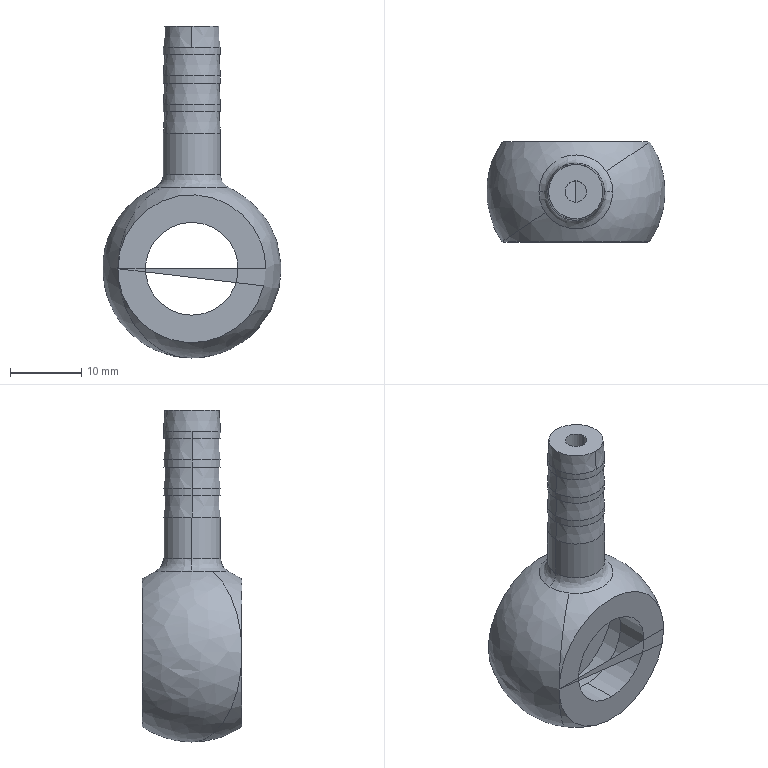Part | SolidWorks | features BaseBody 1 | 1 solid | 37 faces | box 25 x 14 x 46.5 mm | volume 4501 mm3 | cylinder 16 | plane 9 | cone 8 | spline 4 | commonest cylinder face diameters 8 x8 13 x4 3 x2 19 x2
STEP:
#1=CARTESIAN_POINT('',(0.,0.,-12.5));
#2=VERTEX_POINT('',#1);
#3=CARTESIAN_POINT('',(-10.356,-7.,0.));
#4=VERTEX_POINT('',#3);
#5=CARTESIAN_POINT('',(0.,0.,0.));
#6=DIRECTION('',(-0.56,0.8285,0.));
#7=DIRECTION('',(0.,0.,-1.));
#8=AXIS2_PLACEMENT_3D('',#5,#6,#7);
#9=CIRCLE('',#8,12.5);
#10=EDGE_CURVE('',#2,#4,#9,.T.);
#11=ORIENTED_EDGE('',*,*,#10,.F.);
#12=CARTESIAN_POINT('',(10.356,7.,0.));
#13=VERTEX_POINT('',#12);
#14=CARTESIAN_POINT('',(0.,0.,0.));
#15=DIRECTION('',(0.56,-0.8285,0.));
#16=DIRECTION('',(0.,0.,-1.));
#17=AXIS2_PLACEMENT_3D('',#14,#15,#16);
#18=CIRCLE('',#17,12.5);
#19=EDGE_CURVE('',#2,#13,#18,.T.);
#20=ORIENTED_EDGE('',*,*,#19,.T.);
#21=CARTESIAN_POINT('',(4.285,2.897,11.38));
#22=VERTEX_POINT('',#21);
#23=CARTESIAN_POINT('',(0.,0.,0.));
#24=DIRECTION('',(0.56,-0.8285,0.));
#25=DIRECTION('',(0.,0.,-1.));
#26=AXIS2_PLACEMENT_3D('',#23,#24,#25);
#27=CIRCLE('',#26,12.5);
#28=EDGE_CURVE('',#13,#22,#27,.T.);
#29=ORIENTED_EDGE('',*,*,#28,.T.);
#30=CARTESIAN_POINT('',(5.172,-0.000001778,11.38));
#31=VERTEX_POINT('',#30);
#32=CARTESIAN_POINT('',(4.285,2.897,11.38));
#33=CARTESIAN_POINT('',(4.572,2.472,11.38));
#34=CARTESIAN_POINT('',(4.796,2.005,11.38));
#35=CARTESIAN_POINT('',(5.096,1.025,11.38));
#36=CARTESIAN_POINT('',(5.172,0.5124,11.38));
#37=CARTESIAN_POINT('',(5.172,-0.000001778,11.38));
#38=B_SPLINE_CURVE_WITH_KNOTS('',3,(#32,#33,#34,#35,#36,#37),.UNSPECIFIED.,.F.,.F.,(4,2,4),(0.7255,0.8627,1.),.UNSPECIFIED.);
#39=EDGE_CURVE('',#22,#31,#38,.T.);
#40=ORIENTED_EDGE('',*,*,#39,.T.);
#41=CARTESIAN_POINT('',(2.897,-4.285,11.38));
#42=VERTEX_POINT('',#41);
#43=CARTESIAN_POINT('',(0.,0.,11.38));
#44=DIRECTION('',(0.,0.,-1.));
#45=DIRECTION('',(-0.8285,-0.56,0.));
#46=AXIS2_PLACEMENT_3D('',#43,#44,#45);
#47=CIRCLE('',#46,5.172);
#48=EDGE_CURVE('',#31,#42,#47,.T.);
#49=ORIENTED_EDGE('',*,*,#48,.T.);
#50=CARTESIAN_POINT('',(-4.285,-2.897,11.38));
#51=VERTEX_POINT('',#50);
#52=CARTESIAN_POINT('',(2.897,-4.285,11.38));
#53=CARTESIAN_POINT('',(2.336,-4.664,11.38));
#54=CARTESIAN_POINT('',(1.699,-4.932,11.38));
#55=CARTESIAN_POINT('',(0.3728,-5.203,11.38));
#56=CARTESIAN_POINT('',(-0.3172,-5.207,11.38));
#57=CARTESIAN_POINT('',(-1.647,-4.95,11.38));
#58=CARTESIAN_POINT('',(-2.286,-4.689,11.38));
#59=CARTESIAN_POINT('',(-3.416,-3.943,11.38));
#60=CARTESIAN_POINT('',(-3.906,-3.457,11.38));
#61=CARTESIAN_POINT('',(-4.285,-2.897,11.38));
#62=B_SPLINE_CURVE_WITH_KNOTS('',3,(#52,#53,#54,#55,#56,#57,#58,#59,#60,#61),.UNSPECIFIED.,.F.,.F.,(4,2,2,2,4),(0.,0.1814,0.3627,0.5441,0.7255),.UNSPECIFIED.);
#63=EDGE_CURVE('',#42,#51,#62,.T.);
#64=ORIENTED_EDGE('',*,*,#63,.T.);
#65=CARTESIAN_POINT('',(0.,0.,0.));
#66=DIRECTION('',(-0.56,0.8285,0.));
#67=DIRECTION('',(0.,0.,-1.));
#68=AXIS2_PLACEMENT_3D('',#65,#66,#67);
#69=CIRCLE('',#68,12.5);
#70=EDGE_CURVE('',#4,#51,#69,.T.);
#71=ORIENTED_EDGE('',*,*,#70,.F.);
#72=CARTESIAN_POINT('',(10.356,-7.,0.002779));
#73=VERTEX_POINT('',#72);
#74=CARTESIAN_POINT('',(-10.356,-7.,0.));
#75=CARTESIAN_POINT('',(-10.356,-7.,0.6818));
#76=CARTESIAN_POINT('',(-10.289,-7.,1.354));
#77=CARTESIAN_POINT('',(-10.092,-7.,2.347));
#78=CARTESIAN_POINT('',(-10.01,-7.,2.676));
#79=CARTESIAN_POINT('',(-9.813,-7.,3.328));
#80=CARTESIAN_POINT('',(-9.697,-7.,3.651));
#81=CARTESIAN_POINT('',(-9.308,-7.,4.589));
#82=CARTESIAN_POINT('',(-8.991,-7.,5.184));
#83=CARTESIAN_POINT('',(-8.426,-7.,6.03));
#84=CARTESIAN_POINT('',(-8.222,-7.,6.306));
#85=CARTESIAN_POINT('',(-7.79,-7.,6.832));
#86=CARTESIAN_POINT('',(-7.563,-7.,7.083));
#87=CARTESIAN_POINT('',(-6.847,-7.,7.799));
#88=CARTESIAN_POINT('',(-6.326,-7.,8.228));
#89=CARTESIAN_POINT('',(-5.19,-7.,8.988));
#90=CARTESIAN_POINT('',(-4.591,-7.,9.307));
#91=CARTESIAN_POINT('',(-3.657,-7.,9.695));
#92=CARTESIAN_POINT('',(-3.339,-7.,9.809));
#93=CARTESIAN_POINT('',(-2.689,-7.,10.007));
#94=CARTESIAN_POINT('',(-2.356,-7.,10.09));
#95=CARTESIAN_POINT('',(-1.356,-7.,10.289));
#96=CARTESIAN_POINT('',(-0.685,-7.,10.356));
#97=CARTESIAN_POINT('',(0.6675,-7.,10.357));
#98=CARTESIAN_POINT('',(1.354,-7.,10.29));
#99=CARTESIAN_POINT('',(2.68,-7.,10.026));
#100=CARTESIAN_POINT('',(3.326,-7.,9.831));
#101=CARTESIAN_POINT('',(4.269,-7.,9.442));
#102=CARTESIAN_POINT('',(4.579,-7.,9.295));
#103=CARTESIAN_POINT('',(5.181,-7.,8.973));
#104=CARTESIAN_POINT('',(5.472,-7.,8.799));
#105=CARTESIAN_POINT('',(6.314,-7.,8.236));
#106=CARTESIAN_POINT('',(6.837,-7.,7.809));
#107=CARTESIAN_POINT('',(7.56,-7.,7.086));
#108=CARTESIAN_POINT('',(7.79,-7.,6.832));
#109=CARTESIAN_POINT('',(8.22,-7.,6.309));
#110=CARTESIAN_POINT('',(8.622,-7.,5.766));
#111=CARTESIAN_POINT('',(8.97,-7.,5.187));
#112=CARTESIAN_POINT('',(9.29,-7.,4.59));
#113=CARTESIAN_POINT('',(9.436,-7.,4.28));
#114=CARTESIAN_POINT('',(9.828,-7.,3.336));
#115=CARTESIAN_POINT('',(10.023,-7.,2.69));
#116=CARTESIAN_POINT('',(10.222,-7.,1.697));
#117=CARTESIAN_POINT('',(10.272,-7.,1.362));
#118=CARTESIAN_POINT('',(10.339,-7.,0.6824));
#119=CARTESIAN_POINT('',(10.356,-7.,0.3412));
#120=CARTESIAN_POINT('',(10.356,-7.,0.002779));
#121=B_SPLINE_CURVE_WITH_KNOTS('',3,(#74,#75,#76,#77,#78,#79,#80,#81,#82,#83,#84,#85,#86,#87,#88,#89,#90,#91,#92,#93,#94,#95,#96,#97,#98,#99,#100,#101,#102,#103,#104,#105,#106,#107,#108,#109,#110,#111,#112,#113,#114,#115,#116,#117,#118,#119,#120),.UNSPECIFIED.,.F.,.F.,(4,2,2,2,2,2,2,2,2,2,2,2,2,2,2,2,2,2,1,2,2,2,2,4),(0.04367,0.04569,0.0467,0.04771,0.04974,0.05075,0.05176,0.05378,0.05581,0.05682,0.05783,0.05985,0.06188,0.0639,0.06491,0.06592,0.06795,0.06896,0.06997,0.07098,0.07199,0.07402,0.07503,0.07604),.UNSPECIFIED.);
#122=EDGE_CURVE('',#4,#73,#121,.T.);
#123=ORIENTED_EDGE('',*,*,#122,.T.);
#124=CARTESIAN_POINT('',(10.356,-7.,0.002779));
#125=CARTESIAN_POINT('',(10.356,-7.,-0.6741));
#126=CARTESIAN_POINT('',(10.291,-7.,-1.345));
#127=CARTESIAN_POINT('',(10.093,-7.,-2.344));
#128=CARTESIAN_POINT('',(10.01,-7.,-2.677));
#129=CARTESIAN_POINT('',(9.813,-7.,-3.328));
#130=CARTESIAN_POINT('',(9.699,-7.,-3.646));
#131=CARTESIAN_POINT('',(9.312,-7.,-4.582));
#132=CARTESIAN_POINT('',(8.995,-7.,-5.178));
#133=CARTESIAN_POINT('',(8.236,-7.,-6.316));
#134=CARTESIAN_POINT('',(7.806,-7.,-6.839));
#135=CARTESIAN_POINT('',(7.091,-7.,-7.555));
#136=CARTESIAN_POINT('',(6.841,-7.,-7.783));
#137=CARTESIAN_POINT('',(6.316,-7.,-8.214));
#138=CARTESIAN_POINT('',(6.041,-7.,-8.419));
#139=CARTESIAN_POINT('',(5.19,-7.,-8.988));
#140=CARTESIAN_POINT('',(4.583,-7.,-9.312));
#141=CARTESIAN_POINT('',(3.331,-7.,-9.829));
#142=CARTESIAN_POINT('',(2.686,-7.,-10.025));
#143=CARTESIAN_POINT('',(1.688,-7.,-10.223));
#144=CARTESIAN_POINT('',(1.348,-7.,-10.274));
#145=CARTESIAN_POINT('',(0.6714,-7.,-10.34));
#146=CARTESIAN_POINT('',(0.3335,-7.,-10.356));
#147=CARTESIAN_POINT('',(-0.6787,-7.,-10.356));
#148=CARTESIAN_POINT('',(-1.351,-7.,-10.29));
#149=CARTESIAN_POINT('',(-2.692,-7.,-10.023));
#150=CARTESIAN_POINT('',(-3.34,-7.,-9.826));
#151=CARTESIAN_POINT('',(-4.275,-7.,-9.439));
#152=CARTESIAN_POINT('',(-4.581,-7.,-9.294));
#153=CARTESIAN_POINT('',(-5.18,-7.,-8.974));
#154=CARTESIAN_POINT('',(-5.475,-7.,-8.797));
#155=CARTESIAN_POINT('',(-6.321,-7.,-8.231));
#156=CARTESIAN_POINT('',(-6.843,-7.,-7.803));
#157=CARTESIAN_POINT('',(-7.8,-7.,-6.847));
#158=CARTESIAN_POINT('',(-8.237,-7.,-6.313));
#159=CARTESIAN_POINT('',(-8.987,-7.,-5.19));
#160=CARTESIAN_POINT('',(-9.306,-7.,-4.595));
#161=CARTESIAN_POINT('',(-9.697,-7.,-3.652));
#162=CARTESIAN_POINT('',(-9.813,-7.,-3.329));
#163=CARTESIAN_POINT('',(-10.009,-7.,-2.68));
#164=CARTESIAN_POINT('',(-10.173,-7.,-2.024));
#165=CARTESIAN_POINT('',(-10.272,-7.,-1.357));
#166=CARTESIAN_POINT('',(-10.339,-7.,-0.6827));
#167=CARTESIAN_POINT('',(-10.356,-7.,-0.3409));
#168=CARTESIAN_POINT('',(-10.356,-7.,0.));
#169=B_SPLINE_CURVE_WITH_KNOTS('',3,(#124,#125,#126,#127,#128,#129,#130,#131,#132,#133,#134,#135,#136,#137,#138,#139,#140,#141,#142,#143,#144,#145,#146,#147,#148,#149,#150,#151,#152,#153,#154,#155,#156,#157,#158,#159,#160,#161,#162,#163,#164,#165,#166,#167,#168),.UNSPECIFIED.,.F.,.F.,(4,2,2,2,2,2,2,2,2,2,2,2,2,2,2,2,2,2,2,2,1,2,4),(0.01129,0.01332,0.01433,0.01534,0.01736,0.01939,0.0204,0.02141,0.02343,0.02546,0.02647,0.02748,0.0295,0.03153,0.03254,0.03355,0.03557,0.0376,0.03962,0.04063,0.04164,0.04265,0.04367),.UNSPECIFIED.);
#170=EDGE_CURVE('',#73,#4,#169,.T.);
#171=ORIENTED_EDGE('',*,*,#170,.T.);
#172=EDGE_LOOP('',(#11,#20,#29,#40,#49,#64,#71,#123,#171));
#173=FACE_OUTER_BOUND('',#172,.T.);
#174=CARTESIAN_POINT('',(0.,0.,-12.5));
#175=CARTESIAN_POINT('',(0.,0.,-12.5));
#176=CARTESIAN_POINT('',(0.,0.,-12.5));
#177=CARTESIAN_POINT('',(0.,0.,-12.5));
#178=CARTESIAN_POINT('',(0.,0.,-12.5));
#179=CARTESIAN_POINT('',(0.,0.,-12.5));
#180=CARTESIAN_POINT('',(0.,0.,-12.5));
#181=CARTESIAN_POINT('',(14.408,9.738,-12.5));
#182=CARTESIAN_POINT('',(20.112,1.299,-12.5));
#183=CARTESIAN_POINT('',(18.178,-8.703,-12.5));
#184=CARTESIAN_POINT('',(9.738,-14.408,-12.5));
#185=CARTESIAN_POINT('',(1.299,-20.112,-12.5));
#186=CARTESIAN_POINT('',(-8.703,-18.178,-12.5));
#187=CARTESIAN_POINT('',(-14.408,-9.738,-12.5));
#188=CARTESIAN_POINT('',(17.343,11.722,4.525));
#189=CARTESIAN_POINT('',(24.21,1.563,4.525));
#190=CARTESIAN_POINT('',(21.882,-10.476,4.525));
#191=CARTESIAN_POINT('',(11.722,-17.343,4.525));
#192=CARTESIAN_POINT('',(1.563,-24.21,4.525));
#193=CARTESIAN_POINT('',(-10.476,-21.882,4.525));
#194=CARTESIAN_POINT('',(-17.343,-11.722,4.525));
#195=CARTESIAN_POINT('',(4.131,2.792,11.462));
#196=CARTESIAN_POINT('',(5.767,0.3724,11.462));
#197=CARTESIAN_POINT('',(5.212,-2.495,11.462));
#198=CARTESIAN_POINT('',(2.792,-4.131,11.462));
#199=CARTESIAN_POINT('',(0.3724,-5.767,11.462));
#200=CARTESIAN_POINT('',(-2.495,-5.212,11.462));
#201=CARTESIAN_POINT('',(-4.131,-2.792,11.462));
#202=(BOUNDED_SURFACE()B_SPLINE_SURFACE(3,3,((#174,#175,#176,#177,#178,#179,#180),(#181,#182,#183,#184,#185,#186,#187),(#188,#189,#190,#191,#192,#193,#194),(#195,#196,#197,#198,#199,#200,#201)),.UNSPECIFIED.,.F.,.F.,.T.)B_SPLINE_SURFACE_WITH_KNOTS((4,4),(4,3,4),(0.,1.),(0.,0.5,1.),.UNSPECIFIED.)GEOMETRIC_REPRESENTATION_ITEM()RATIONAL_B_SPLINE_SURFACE(((1.,0.8047,0.8047,1.,0.8047,0.8047,1.),(0.4692,0.3775,0.3775,0.4692,0.3775,0.3775,0.4692),(0.4692,0.3775,0.3775,0.4692,0.3775,0.3775,0.4692),(1.,0.8047,0.8047,1.,0.8047,0.8047,1.)))REPRESENTATION_ITEM('')SURFACE());
#203=ADVANCED_FACE('',(#173),#202,.T.);
#204=CARTESIAN_POINT('',(-4.,0.,19.));
#205=VERTEX_POINT('',#204);
#206=CARTESIAN_POINT('',(4.,0.,19.));
#207=VERTEX_POINT('',#206);
#208=CARTESIAN_POINT('',(0.,0.,19.));
#209=DIRECTION('',(0.,0.,-1.));
#210=DIRECTION('',(-1.,0.,0.));
#211=AXIS2_PLACEMENT_3D('',#208,#209,#210);
#212=CIRCLE('',#211,4.);
#213=EDGE_CURVE('',#205,#207,#212,.T.);
#214=ORIENTED_EDGE('',*,*,#213,.T.);
#215=CARTESIAN_POINT('',(4.,-0.000001036,13.2));
#216=VERTEX_POINT('',#215);
#217=CARTESIAN_POINT('',(4.,0.,19.));
#218=DIRECTION('',(0.,0.,-1.));
#219=VECTOR('',#218,1000.);
#220=LINE('',#217,#219);
#221=EDGE_CURVE('',#207,#216,#220,.T.);
#222=ORIENTED_EDGE('',*,*,#221,.T.);
#223=CARTESIAN_POINT('',(-4.,0.000000641,13.2));
#224=VERTEX_POINT('',#223);
#225=CARTESIAN_POINT('',(-0.000000135,-0.000000379,13.2));
#226=DIRECTION('',(0.000000022,0.00000006,1.));
#227=DIRECTION('',(1.,-0.000000251,-0.000000022));
#228=AXIS2_PLACEMENT_3D('',#225,#226,#227);
#229=CIRCLE('',#228,4.);
#230=EDGE_CURVE('',#216,#224,#229,.T.);
#231=ORIENTED_EDGE('',*,*,#230,.T.);
#232=CARTESIAN_POINT('',(-4.,0.,19.));
#233=DIRECTION('',(0.,0.,-1.));
#234=VECTOR('',#233,1000.);
#235=LINE('',#232,#234);
#236=EDGE_CURVE('',#205,#224,#235,.T.);
#237=ORIENTED_EDGE('',*,*,#236,.F.);
#238=EDGE_LOOP('',(#214,#222,#231,#237));
#239=FACE_OUTER_BOUND('',#238,.T.);
#240=CARTESIAN_POINT('',(0.,0.,19.));
#241=DIRECTION('',(0.,0.,-1.));
#242=DIRECTION('',(-1.,0.,0.));
#243=AXIS2_PLACEMENT_3D('',#240,#241,#242);
#244=CYLINDRICAL_SURFACE('',#243,4.);
#245=ADVANCED_FACE('',(#239),#244,.T.);
#246=CARTESIAN_POINT('',(0.,7.,6.5));
#247=VERTEX_POINT('',#246);
#248=CARTESIAN_POINT('',(0.,7.,-6.5));
#249=VERTEX_POINT('',#248);
#250=CARTESIAN_POINT('',(0.,7.,0.));
#251=DIRECTION('',(0.,-1.,0.));
#252=DIRECTION('',(0.,0.,-1.));
#253=AXIS2_PLACEMENT_3D('',#250,#251,#252);
#254=CIRCLE('',#253,6.5);
#255=EDGE_CURVE('',#247,#249,#254,.T.);
#256=ORIENTED_EDGE('',*,*,#255,.F.);
#257=CARTESIAN_POINT('',(0.,2.333,6.5));
#258=VERTEX_POINT('',#257);
#259=CARTESIAN_POINT('',(0.,7.,6.5));
#260=DIRECTION('',(0.,-1.,0.));
#261=VECTOR('',#260,1000.);
#262=LINE('',#259,#261);
#263=EDGE_CURVE('',#247,#258,#262,.T.);
#264=ORIENTED_EDGE('',*,*,#263,.T.);
#265=CARTESIAN_POINT('',(0.,2.333,-6.5));
#266=VERTEX_POINT('',#265);
#267=CARTESIAN_POINT('',(0.,2.333,0.));
#268=DIRECTION('',(0.,1.,0.));
#269=DIRECTION('',(0.,0.,-1.));
#270=AXIS2_PLACEMENT_3D('',#267,#268,#269);
#271=CIRCLE('',#270,6.5);
#272=EDGE_CURVE('',#266,#258,#271,.T.);
#273=ORIENTED_EDGE('',*,*,#272,.F.);
#274=CARTESIAN_POINT('',(0.,7.,-6.5));
#275=DIRECTION('',(0.,-1.,0.));
#276=VECTOR('',#275,1000.);
#277=LINE('',#274,#276);
#278=EDGE_CURVE('',#249,#266,#277,.T.);
#279=ORIENTED_EDGE('',*,*,#278,.F.);
#280=EDGE_LOOP('',(#256,#264,#273,#279));
#281=FACE_OUTER_BOUND('',#280,.T.);
#282=CARTESIAN_POINT('',(0.,7.,0.));
#283=DIRECTION('',(0.,-1.,0.));
#284=DIRECTION('',(0.,0.,-1.));
#285=AXIS2_PLACEMENT_3D('',#282,#283,#284);
#286=CYLINDRICAL_SURFACE('',#285,6.5);
#287=ADVANCED_FACE('',(#281),#286,.F.);
#288=CARTESIAN_POINT('',(0.,-2.333,6.5));
#289=VERTEX_POINT('',#288);
#290=CARTESIAN_POINT('',(0.,-2.333,-6.5));
#291=VERTEX_POINT('',#290);
#292=CARTESIAN_POINT('',(0.,-2.333,0.));
#293=DIRECTION('',(0.,-1.,0.));
#294=DIRECTION('',(0.,0.,-1.));
#295=AXIS2_PLACEMENT_3D('',#292,#293,#294);
#296=CIRCLE('',#295,6.5);
#297=EDGE_CURVE('',#289,#291,#296,.T.);
#298=ORIENTED_EDGE('',*,*,#297,.F.);
#299=CARTESIAN_POINT('',(0.,-7.,6.5));
#300=VERTEX_POINT('',#299);
#301=CARTESIAN_POINT('',(0.,-2.333,6.5));
#302=DIRECTION('',(0.,-1.,0.));
#303=VECTOR('',#302,1000.);
#304=LINE('',#301,#303);
#305=EDGE_CURVE('',#289,#300,#304,.T.);
#306=ORIENTED_EDGE('',*,*,#305,.T.);
#307=CARTESIAN_POINT('',(0.,-7.,-6.5));
#308=VERTEX_POINT('',#307);
#309=CARTESIAN_POINT('',(0.,-7.,0.));
#310=DIRECTION('',(0.,-1.,0.));
#311=DIRECTION('',(0.,0.,-1.));
#312=AXIS2_PLACEMENT_3D('',#309,#310,#311);
#313=CIRCLE('',#312,6.5);
#314=EDGE_CURVE('',#300,#308,#313,.T.);
#315=ORIENTED_EDGE('',*,*,#314,.T.);
#316=CARTESIAN_POINT('',(0.,-2.333,-6.5));
#317=DIRECTION('',(0.,-1.,0.));
#318=VECTOR('',#317,1000.);
#319=LINE('',#316,#318);
#320=EDGE_CURVE('',#291,#308,#319,.T.);
#321=ORIENTED_EDGE('',*,*,#320,.F.);
#322=EDGE_LOOP('',(#298,#306,#315,#321));
#323=FACE_OUTER_BOUND('',#322,.T.);
#324=CARTESIAN_POINT('',(0.,-2.333,0.));
#325=DIRECTION('',(0.,-1.,0.));
#326=DIRECTION('',(0.,0.,-1.));
#327=AXIS2_PLACEMENT_3D('',#324,#325,#326);
#328=CYLINDRICAL_SURFACE('',#327,6.5);
#329=ADVANCED_FACE('',(#323),#328,.F.);
#330=CARTESIAN_POINT('',(-3.8,0.,22.));
#331=VERTEX_POINT('',#330);
#332=CARTESIAN_POINT('',(3.8,0.,22.));
#333=VERTEX_POINT('',#332);
#334=CARTESIAN_POINT('',(0.,0.,22.));
#335=DIRECTION('',(0.,0.,-1.));
#336=DIRECTION('',(-1.,0.,0.));
#337=AXIS2_PLACEMENT_3D('',#334,#335,#336);
#338=CIRCLE('',#337,3.8);
#339=EDGE_CURVE('',#331,#333,#338,.T.);
#340=ORIENTED_EDGE('',*,*,#339,.T.);
#341=CARTESIAN_POINT('',(4.,0.,19.));
#342=DIRECTION('',(0.06652,0.,-0.9978));
#343=VECTOR('',#342,1000.);
#344=LINE('',#341,#343);
#345=EDGE_CURVE('',#333,#207,#344,.T.);
#346=ORIENTED_EDGE('',*,*,#345,.T.);
#347=ORIENTED_EDGE('',*,*,#213,.F.);
#348=CARTESIAN_POINT('',(-4.,0.,19.));
#349=DIRECTION('',(-0.06652,0.,-0.9978));
#350=VECTOR('',#349,1000.);
#351=LINE('',#348,#350);
#352=EDGE_CURVE('',#331,#205,#351,.T.);
#353=ORIENTED_EDGE('',*,*,#352,.F.);
#354=EDGE_LOOP('',(#340,#346,#347,#353));
#355=FACE_OUTER_BOUND('',#354,.T.);
#356=CARTESIAN_POINT('',(0.,0.,19.));
#357=DIRECTION('',(0.,0.,-1.));
#358=DIRECTION('',(-1.,0.,0.));
#359=AXIS2_PLACEMENT_3D('',#356,#357,#358);
#360=CONICAL_SURFACE('',#359,4.,0.06657);
#361=ADVANCED_FACE('',(#355),#360,.T.);
#362=CARTESIAN_POINT('',(3.041,2.333,9.));
#363=VERTEX_POINT('',#362);
#364=CARTESIAN_POINT('',(0.,2.333,-9.5));
#365=VERTEX_POINT('',#364);
#366=CARTESIAN_POINT('',(0.,2.333,0.));
#367=DIRECTION('',(0.,1.,0.));
#368=DIRECTION('',(0.,0.,-1.));
#369=AXIS2_PLACEMENT_3D('',#366,#367,#368);
#370=CIRCLE('',#369,9.5);
#371=EDGE_CURVE('',#363,#365,#370,.T.);
#372=ORIENTED_EDGE('',*,*,#371,.T.);
#373=CARTESIAN_POINT('',(0.,-2.333,-9.5));
#374=VERTEX_POINT('',#373);
#375=CARTESIAN_POINT('',(0.,2.333,-9.5));
#376=DIRECTION('',(0.,-1.,0.));
#377=VECTOR('',#376,1000.);
#378=LINE('',#375,#377);
#379=EDGE_CURVE('',#365,#374,#378,.T.);
#380=ORIENTED_EDGE('',*,*,#379,.T.);
#381=CARTESIAN_POINT('',(3.041,-2.333,9.));
#382=VERTEX_POINT('',#381);
#383=CARTESIAN_POINT('',(0.,-2.333,0.));
#384=DIRECTION('',(0.,1.,0.));
#385=DIRECTION('',(0.,0.,-1.));
#386=AXIS2_PLACEMENT_3D('',#383,#384,#385);
#387=CIRCLE('',#386,9.5);
#388=EDGE_CURVE('',#382,#374,#387,.T.);
#389=ORIENTED_EDGE('',*,*,#388,.F.);
#390=CARTESIAN_POINT('',(3.041,2.333,9.));
#391=DIRECTION('',(0.,-1.,0.));
#392=VECTOR('',#391,1000.);
#393=LINE('',#390,#392);
#394=EDGE_CURVE('',#363,#382,#393,.T.);
#395=ORIENTED_EDGE('',*,*,#394,.F.);
#396=EDGE_LOOP('',(#372,#380,#389,#395));
#397=FACE_OUTER_BOUND('',#396,.T.);
#398=CARTESIAN_POINT('',(0.,2.333,0.));
#399=DIRECTION('',(0.,-1.,0.));
#400=DIRECTION('',(0.,0.,-1.));
#401=AXIS2_PLACEMENT_3D('',#398,#399,#400);
#402=CYLINDRICAL_SURFACE('',#401,9.5);
#403=ADVANCED_FACE('',(#397),#402,.F.);
#404=CARTESIAN_POINT('',(-4.,0.,23.));
#405=VERTEX_POINT('',#404);
#406=CARTESIAN_POINT('',(4.,0.,23.));
#407=VERTEX_POINT('',#406);
#408=CARTESIAN_POINT('',(0.,0.,23.));
#409=DIRECTION('',(0.,0.,-1.));
#410=DIRECTION('',(-1.,0.,0.));
#411=AXIS2_PLACEMENT_3D('',#408,#409,#410);
#412=CIRCLE('',#411,4.);
#413=EDGE_CURVE('',#405,#407,#412,.T.);
#414=ORIENTED_EDGE('',*,*,#413,.T.);
#415=CARTESIAN_POINT('',(4.,0.,22.));
#416=VERTEX_POINT('',#415);
#417=CARTESIAN_POINT('',(4.,0.,23.));
#418=DIRECTION('',(0.,0.,-1.));
#419=VECTOR('',#418,1000.);
#420=LINE('',#417,#419);
#421=EDGE_CURVE('',#407,#416,#420,.T.);
#422=ORIENTED_EDGE('',*,*,#421,.T.);
#423=CARTESIAN_POINT('',(-4.,0.,22.));
#424=VERTEX_POINT('',#423);
#425=CARTESIAN_POINT('',(0.,0.,22.));
#426=DIRECTION('',(0.,0.,1.));
#427=DIRECTION('',(-1.,0.,0.));
#428=AXIS2_PLACEMENT_3D('',#425,#426,#427);
#429=CIRCLE('',#428,4.);
#430=EDGE_CURVE('',#416,#424,#429,.T.);
#431=ORIENTED_EDGE('',*,*,#430,.T.);
#432=CARTESIAN_POINT('',(-4.,0.,23.));
#433=DIRECTION('',(0.,0.,-1.));
#434=VECTOR('',#433,1000.);
#435=LINE('',#432,#434);
#436=EDGE_CURVE('',#405,#424,#435,.T.);
#437=ORIENTED_EDGE('',*,*,#436,.F.);
#438=EDGE_LOOP('',(#414,#422,#431,#437));
#439=FACE_OUTER_BOUND('',#438,.T.);
#440=CARTESIAN_POINT('',(0.,0.,23.));
#441=DIRECTION('',(0.,0.,-1.));
#442=DIRECTION('',(-1.,0.,0.));
#443=AXIS2_PLACEMENT_3D('',#440,#441,#442);
#444=CYLINDRICAL_SURFACE('',#443,4.);
#445=ADVANCED_FACE('',(#439),#444,.T.);
#446=CARTESIAN_POINT('',(1.5,0.,34.));
#447=VERTEX_POINT('',#446);
#448=CARTESIAN_POINT('',(-1.5,0.,34.));
#449=VERTEX_POINT('',#448);
#450=CARTESIAN_POINT('',(0.,0.,34.));
#451=DIRECTION('',(0.,0.,-1.));
#452=DIRECTION('',(-1.,0.,0.));
#453=AXIS2_PLACEMENT_3D('',#450,#451,#452);
#454=CIRCLE('',#453,1.5);
#455=EDGE_CURVE('',#447,#449,#454,.T.);
#456=ORIENTED_EDGE('',*,*,#455,.F.);
#457=CARTESIAN_POINT('',(1.5,0.,9.));
#458=VERTEX_POINT('',#457);
#459=CARTESIAN_POINT('',(1.5,0.,34.));
#460=DIRECTION('',(0.,0.,-1.));
#461=VECTOR('',#460,1000.);
#462=LINE('',#459,#461);
#463=EDGE_CURVE('',#447,#458,#462,.T.);
#464=ORIENTED_EDGE('',*,*,#463,.T.);
#465=CARTESIAN_POINT('',(-1.5,0.,9.));
#466=VERTEX_POINT('',#465);
#467=CARTESIAN_POINT('',(0.,0.,9.));
#468=DIRECTION('',(0.,0.,-1.));
#469=DIRECTION('',(-1.,0.,0.));
#470=AXIS2_PLACEMENT_3D('',#467,#468,#469);
#471=CIRCLE('',#470,1.5);
#472=EDGE_CURVE('',#458,#466,#471,.T.);
#473=ORIENTED_EDGE('',*,*,#472,.T.);
#474=CARTESIAN_POINT('',(-1.5,0.,34.));
#475=DIRECTION('',(0.,0.,-1.));
#476=VECTOR('',#475,1000.);
#477=LINE('',#474,#476);
#478=EDGE_CURVE('',#449,#466,#477,.T.);
#479=ORIENTED_EDGE('',*,*,#478,.F.);
#480=EDGE_LOOP('',(#456,#464,#473,#479));
#481=FACE_OUTER_BOUND('',#480,.T.);
#482=CARTESIAN_POINT('',(0.,0.,34.));
#483=DIRECTION('',(0.,0.,-1.));
#484=DIRECTION('',(-1.,0.,0.));
#485=AXIS2_PLACEMENT_3D('',#482,#483,#484);
#486=CYLINDRICAL_SURFACE('',#485,1.5);
#487=ADVANCED_FACE('',(#481),#486,.F.);
#488=CARTESIAN_POINT('',(-3.8,0.,26.));
#489=VERTEX_POINT('',#488);
#490=CARTESIAN_POINT('',(3.8,0.,26.));
#491=VERTEX_POINT('',#490);
#492=CARTESIAN_POINT('',(0.,0.,26.));
#493=DIRECTION('',(0.,0.,-1.));
#494=DIRECTION('',(-1.,0.,0.));
#495=AXIS2_PLACEMENT_3D('',#492,#493,#494);
#496=CIRCLE('',#495,3.8);
#497=EDGE_CURVE('',#489,#491,#496,.T.);
#498=ORIENTED_EDGE('',*,*,#497,.T.);
#499=CARTESIAN_POINT('',(4.,0.,23.));
#500=DIRECTION('',(0.06652,0.,-0.9978));
#501=VECTOR('',#500,1000.);
#502=LINE('',#499,#501);
#503=EDGE_CURVE('',#491,#407,#502,.T.);
#504=ORIENTED_EDGE('',*,*,#503,.T.);
#505=ORIENTED_EDGE('',*,*,#413,.F.);
#506=CARTESIAN_POINT('',(-4.,0.,23.));
#507=DIRECTION('',(-0.06652,0.,-0.9978));
#508=VECTOR('',#507,1000.);
#509=LINE('',#506,#508);
#510=EDGE_CURVE('',#489,#405,#509,.T.);
#511=ORIENTED_EDGE('',*,*,#510,.F.);
#512=EDGE_LOOP('',(#498,#504,#505,#511));
#513=FACE_OUTER_BOUND('',#512,.T.);
#514=CARTESIAN_POINT('',(0.,0.,23.));
#515=DIRECTION('',(0.,0.,-1.));
#516=DIRECTION('',(-1.,0.,0.));
#517=AXIS2_PLACEMENT_3D('',#514,#515,#516);
#518=CONICAL_SURFACE('',#517,4.,0.06657);
#519=ADVANCED_FACE('',(#513),#518,.T.);
#520=CARTESIAN_POINT('',(0.,-3.8,34.));
#521=VERTEX_POINT('',#520);
#522=CARTESIAN_POINT('',(0.,3.8,34.));
#523=VERTEX_POINT('',#522);
#524=CARTESIAN_POINT('',(0.,0.,34.));
#525=DIRECTION('',(0.,0.,1.));
#526=DIRECTION('',(0.,1.,0.));
#527=AXIS2_PLACEMENT_3D('',#524,#525,#526);
#528=CIRCLE('',#527,3.8);
#529=EDGE_CURVE('',#521,#523,#528,.T.);
#530=ORIENTED_EDGE('',*,*,#529,.F.);
#531=CARTESIAN_POINT('',(0.,-4.,31.));
#532=VERTEX_POINT('',#531);
#533=CARTESIAN_POINT('',(0.,-4.,31.));
#534=DIRECTION('',(0.,-0.06652,-0.9978));
#535=VECTOR('',#534,1000.);
#536=LINE('',#533,#535);
#537=EDGE_CURVE('',#521,#532,#536,.T.);
#538=ORIENTED_EDGE('',*,*,#537,.T.);
#539=CARTESIAN_POINT('',(4.,0.,31.));
#540=VERTEX_POINT('',#539);
#541=CARTESIAN_POINT('',(0.,0.,31.));
#542=DIRECTION('',(0.,0.,1.));
#543=DIRECTION('',(-1.,0.,0.));
#544=AXIS2_PLACEMENT_3D('',#541,#542,#543);
#545=CIRCLE('',#544,4.);
#546=EDGE_CURVE('',#532,#540,#545,.T.);
#547=ORIENTED_EDGE('',*,*,#546,.T.);
#548=CARTESIAN_POINT('',(0.,4.,31.));
#549=VERTEX_POINT('',#548);
#550=CARTESIAN_POINT('',(0.,0.,31.));
#551=DIRECTION('',(0.,0.,1.));
#552=DIRECTION('',(-1.,0.,0.));
#553=AXIS2_PLACEMENT_3D('',#550,#551,#552);
#554=CIRCLE('',#553,4.);
#555=EDGE_CURVE('',#540,#549,#554,.T.);
#556=ORIENTED_EDGE('',*,*,#555,.T.);
#557=CARTESIAN_POINT('',(0.,4.,31.));
#558=DIRECTION('',(0.,0.06652,-0.9978));
#559=VECTOR('',#558,1000.);
#560=LINE('',#557,#559);
#561=EDGE_CURVE('',#523,#549,#560,.T.);
#562=ORIENTED_EDGE('',*,*,#561,.F.);
#563=EDGE_LOOP('',(#530,#538,#547,#556,#562));
#564=FACE_OUTER_BOUND('',#563,.T.);
#565=CARTESIAN_POINT('',(0.,0.,31.));
#566=DIRECTION('',(0.,0.,-1.));
#567=DIRECTION('',(0.,1.,0.));
#568=AXIS2_PLACEMENT_3D('',#565,#566,#567);
#569=CONICAL_SURFACE('',#568,4.,0.06657);
#570=ADVANCED_FACE('',(#564),#569,.T.);
#571=CARTESIAN_POINT('',(-4.,0.,27.));
#572=VERTEX_POINT('',#571);
#573=CARTESIAN_POINT('',(4.,0.,27.));
#574=VERTEX_POINT('',#573);
#575=CARTESIAN_POINT('',(0.,0.,27.));
#576=DIRECTION('',(0.,0.,-1.));
#577=DIRECTION('',(-1.,0.,0.));
#578=AXIS2_PLACEMENT_3D('',#575,#576,#577);
#579=CIRCLE('',#578,4.);
#580=EDGE_CURVE('',#572,#574,#579,.T.);
#581=ORIENTED_EDGE('',*,*,#580,.T.);
#582=CARTESIAN_POINT('',(4.,0.,26.));
#583=VERTEX_POINT('',#582);
#584=CARTESIAN_POINT('',(4.,0.,27.));
#585=DIRECTION('',(0.,0.,-1.));
#586=VECTOR('',#585,1000.);
#587=LINE('',#584,#586);
#588=EDGE_CURVE('',#574,#583,#587,.T.);
#589=ORIENTED_EDGE('',*,*,#588,.T.);
#590=CARTESIAN_POINT('',(-4.,0.,26.));
#591=VERTEX_POINT('',#590);
#592=CARTESIAN_POINT('',(0.,0.,26.));
#593=DIRECTION('',(0.,0.,1.));
#594=DIRECTION('',(-1.,0.,0.));
#595=AXIS2_PLACEMENT_3D('',#592,#593,#594);
#596=CIRCLE('',#595,4.);
#597=EDGE_CURVE('',#583,#591,#596,.T.);
#598=ORIENTED_EDGE('',*,*,#597,.T.);
#599=CARTESIAN_POINT('',(-4.,0.,27.));
#600=DIRECTION('',(0.,0.,-1.));
#601=VECTOR('',#600,1000.);
#602=LINE('',#599,#601);
#603=EDGE_CURVE('',#572,#591,#602,.T.);
#604=ORIENTED_EDGE('',*,*,#603,.F.);
#605=EDGE_LOOP('',(#581,#589,#598,#604));
#606=FACE_OUTER_BOUND('',#605,.T.);
#607=CARTESIAN_POINT('',(0.,0.,27.));
#608=DIRECTION('',(0.,0.,-1.));
#609=DIRECTION('',(-1.,0.,0.));
#610=AXIS2_PLACEMENT_3D('',#607,#608,#609);
#611=CYLINDRICAL_SURFACE('',#610,4.);
#612=ADVANCED_FACE('',(#606),#611,.T.);
#613=ORIENTED_EDGE('',*,*,#555,.F.);
#614=CARTESIAN_POINT('',(4.,0.,30.));
#615=VERTEX_POINT('',#614);
#616=CARTESIAN_POINT('',(4.,0.,31.));
#617=DIRECTION('',(0.,0.,-1.));
#618=VECTOR('',#617,1000.);
#619=LINE('',#616,#618);
#620=EDGE_CURVE('',#540,#615,#619,.T.);
#621=ORIENTED_EDGE('',*,*,#620,.T.);
#622=CARTESIAN_POINT('',(-4.,0.,30.));
#623=VERTEX_POINT('',#622);
#624=CARTESIAN_POINT('',(0.,0.,30.));
#625=DIRECTION('',(0.,0.,1.));
#626=DIRECTION('',(-1.,0.,0.));
#627=AXIS2_PLACEMENT_3D('',#624,#625,#626);
#628=CIRCLE('',#627,4.);
#629=EDGE_CURVE('',#615,#623,#628,.T.);
#630=ORIENTED_EDGE('',*,*,#629,.T.);
#631=CARTESIAN_POINT('',(-4.,0.,31.));
#632=VERTEX_POINT('',#631);
#633=CARTESIAN_POINT('',(-4.,0.,31.));
#634=DIRECTION('',(0.,0.,-1.));
#635=VECTOR('',#634,1000.);
#636=LINE('',#633,#635);
#637=EDGE_CURVE('',#632,#623,#636,.T.);
#638=ORIENTED_EDGE('',*,*,#637,.F.);
#639=CARTESIAN_POINT('',(0.,0.,31.));
#640=DIRECTION('',(0.,0.,1.));
#641=DIRECTION('',(-1.,0.,0.));
#642=AXIS2_PLACEMENT_3D('',#639,#640,#641);
#643=CIRCLE('',#642,4.);
#644=EDGE_CURVE('',#549,#632,#643,.T.);
#645=ORIENTED_EDGE('',*,*,#644,.F.);
#646=EDGE_LOOP('',(#613,#621,#630,#638,#645));
#647=FACE_OUTER_BOUND('',#646,.T.);
#648=CARTESIAN_POINT('',(0.,0.,31.));
#649=DIRECTION('',(0.,0.,-1.));
#650=DIRECTION('',(-1.,0.,0.));
#651=AXIS2_PLACEMENT_3D('',#648,#649,#650);
#652=CYLINDRICAL_SURFACE('',#651,4.);
#653=ADVANCED_FACE('',(#647),#652,.T.);
#654=CARTESIAN_POINT('',(-3.8,0.,30.));
#655=VERTEX_POINT('',#654);
#656=CARTESIAN_POINT('',(3.8,0.,30.));
#657=VERTEX_POINT('',#656);
#658=CARTESIAN_POINT('',(0.,0.,30.));
#659=DIRECTION('',(0.,0.,-1.));
#660=DIRECTION('',(-1.,0.,0.));
#661=AXIS2_PLACEMENT_3D('',#658,#659,#660);
#662=CIRCLE('',#661,3.8);
#663=EDGE_CURVE('',#655,#657,#662,.T.);
#664=ORIENTED_EDGE('',*,*,#663,.T.);
#665=CARTESIAN_POINT('',(4.,0.,27.));
#666=DIRECTION('',(0.06652,0.,-0.9978));
#667=VECTOR('',#666,1000.);
#668=LINE('',#665,#667);
#669=EDGE_CURVE('',#657,#574,#668,.T.);
#670=ORIENTED_EDGE('',*,*,#669,.T.);
#671=ORIENTED_EDGE('',*,*,#580,.F.);
#672=CARTESIAN_POINT('',(-4.,0.,27.));
#673=DIRECTION('',(-0.06652,0.,-0.9978));
#674=VECTOR('',#673,1000.);
#675=LINE('',#672,#674);
#676=EDGE_CURVE('',#655,#572,#675,.T.);
#677=ORIENTED_EDGE('',*,*,#676,.F.);
#678=EDGE_LOOP('',(#664,#670,#671,#677));
#679=FACE_OUTER_BOUND('',#678,.T.);
#680=CARTESIAN_POINT('',(0.,0.,27.));
#681=DIRECTION('',(0.,0.,-1.));
#682=DIRECTION('',(-1.,0.,0.));
#683=AXIS2_PLACEMENT_3D('',#680,#681,#682);
#684=CONICAL_SURFACE('',#683,4.,0.06657);
#685=ADVANCED_FACE('',(#679),#684,.T.);
#686=ORIENTED_EDGE('',*,*,#19,.F.);
#687=ORIENTED_EDGE('',*,*,#10,.T.);
#688=ORIENTED_EDGE('',*,*,#70,.T.);
#689=CARTESIAN_POINT('',(-5.172,0.000000275,11.38));
#690=VERTEX_POINT('',#689);
#691=CARTESIAN_POINT('',(-4.285,-2.897,11.38));
#692=CARTESIAN_POINT('',(-4.572,-2.472,11.38));
#693=CARTESIAN_POINT('',(-4.796,-2.005,11.38));
#694=CARTESIAN_POINT('',(-5.096,-1.025,11.38));
#695=CARTESIAN_POINT('',(-5.172,-0.5124,11.38));
#696=CARTESIAN_POINT('',(-5.172,0.000000275,11.38));
#697=B_SPLINE_CURVE_WITH_KNOTS('',3,(#691,#692,#693,#694,#695,#696),.UNSPECIFIED.,.F.,.F.,(4,2,4),(0.7255,0.8627,1.),.UNSPECIFIED.);
#698=EDGE_CURVE('',#51,#690,#697,.T.);
#699=ORIENTED_EDGE('',*,*,#698,.T.);
#700=CARTESIAN_POINT('',(-2.897,4.285,11.38));
#701=VERTEX_POINT('',#700);
#702=CARTESIAN_POINT('',(-0.000000175,-0.000000488,11.38));
#703=DIRECTION('',(-0.000000022,-0.00000006,-1.));
#704=DIRECTION('',(1.,-0.000000251,-0.000000022));
#705=AXIS2_PLACEMENT_3D('',#702,#703,#704);
#706=CIRCLE('',#705,5.172);
#707=EDGE_CURVE('',#690,#701,#706,.T.);
#708=ORIENTED_EDGE('',*,*,#707,.T.);
#709=CARTESIAN_POINT('',(-2.897,4.285,11.38));
#710=CARTESIAN_POINT('',(-2.336,4.664,11.38));
#711=CARTESIAN_POINT('',(-1.699,4.932,11.38));
#712=CARTESIAN_POINT('',(-0.3728,5.203,11.38));
#713=CARTESIAN_POINT('',(0.3172,5.207,11.38));
#714=CARTESIAN_POINT('',(1.647,4.95,11.38));
#715=CARTESIAN_POINT('',(2.286,4.689,11.38));
#716=CARTESIAN_POINT('',(3.416,3.943,11.38));
#717=CARTESIAN_POINT('',(3.906,3.457,11.38));
#718=CARTESIAN_POINT('',(4.285,2.897,11.38));
#719=B_SPLINE_CURVE_WITH_KNOTS('',3,(#709,#710,#711,#712,#713,#714,#715,#716,#717,#718),.UNSPECIFIED.,.F.,.F.,(4,2,2,2,4),(0.,0.1814,0.3627,0.5441,0.7255),.UNSPECIFIED.);
#720=EDGE_CURVE('',#701,#22,#719,.T.);
#721=ORIENTED_EDGE('',*,*,#720,.T.);
#722=ORIENTED_EDGE('',*,*,#28,.F.);
#723=CARTESIAN_POINT('',(-10.356,7.,0.002779));
#724=VERTEX_POINT('',#723);
#725=CARTESIAN_POINT('',(10.356,7.,0.));
#726=CARTESIAN_POINT('',(10.356,7.,0.6818));
#727=CARTESIAN_POINT('',(10.289,7.,1.354));
#728=CARTESIAN_POINT('',(10.092,7.,2.347));
#729=CARTESIAN_POINT('',(10.01,7.,2.676));
#730=CARTESIAN_POINT('',(9.813,7.,3.328));
#731=CARTESIAN_POINT('',(9.697,7.,3.651));
#732=CARTESIAN_POINT('',(9.308,7.,4.589));
#733=CARTESIAN_POINT('',(8.991,7.,5.184));
#734=CARTESIAN_POINT('',(8.426,7.,6.03));
#735=CARTESIAN_POINT('',(8.222,7.,6.306));
#736=CARTESIAN_POINT('',(7.79,7.,6.832));
#737=CARTESIAN_POINT('',(7.563,7.,7.083));
#738=CARTESIAN_POINT('',(6.847,7.,7.799));
#739=CARTESIAN_POINT('',(6.326,7.,8.228));
#740=CARTESIAN_POINT('',(5.19,7.,8.988));
#741=CARTESIAN_POINT('',(4.591,7.,9.307));
#742=CARTESIAN_POINT('',(3.657,7.,9.695));
#743=CARTESIAN_POINT('',(3.339,7.,9.809));
#744=CARTESIAN_POINT('',(2.689,7.,10.007));
#745=CARTESIAN_POINT('',(2.356,7.,10.09));
#746=CARTESIAN_POINT('',(1.356,7.,10.289));
#747=CARTESIAN_POINT('',(0.685,7.,10.356));
#748=CARTESIAN_POINT('',(-0.6675,7.,10.357));
#749=CARTESIAN_POINT('',(-1.354,7.,10.29));
#750=CARTESIAN_POINT('',(-2.68,7.,10.026));
#751=CARTESIAN_POINT('',(-3.326,7.,9.831));
#752=CARTESIAN_POINT('',(-4.269,7.,9.442));
#753=CARTESIAN_POINT('',(-4.579,7.,9.295));
#754=CARTESIAN_POINT('',(-5.181,7.,8.973));
#755=CARTESIAN_POINT('',(-5.472,7.,8.799));
#756=CARTESIAN_POINT('',(-6.314,7.,8.236));
#757=CARTESIAN_POINT('',(-6.837,7.,7.809));
#758=CARTESIAN_POINT('',(-7.56,7.,7.086));
#759=CARTESIAN_POINT('',(-7.79,7.,6.832));
#760=CARTESIAN_POINT('',(-8.22,7.,6.309));
#761=CARTESIAN_POINT('',(-8.622,7.,5.766));
#762=CARTESIAN_POINT('',(-8.97,7.,5.187));
#763=CARTESIAN_POINT('',(-9.29,7.,4.59));
#764=CARTESIAN_POINT('',(-9.436,7.,4.28));
#765=CARTESIAN_POINT('',(-9.828,7.,3.336));
#766=CARTESIAN_POINT('',(-10.023,7.,2.69));
#767=CARTESIAN_POINT('',(-10.222,7.,1.697));
#768=CARTESIAN_POINT('',(-10.272,7.,1.362));
#769=CARTESIAN_POINT('',(-10.339,7.,0.6824));
#770=CARTESIAN_POINT('',(-10.356,7.,0.3412));
#771=CARTESIAN_POINT('',(-10.356,7.,0.002779));
#772=B_SPLINE_CURVE_WITH_KNOTS('',3,(#725,#726,#727,#728,#729,#730,#731,#732,#733,#734,#735,#736,#737,#738,#739,#740,#741,#742,#743,#744,#745,#746,#747,#748,#749,#750,#751,#752,#753,#754,#755,#756,#757,#758,#759,#760,#761,#762,#763,#764,#765,#766,#767,#768,#769,#770,#771),.UNSPECIFIED.,.F.,.F.,(4,2,2,2,2,2,2,2,2,2,2,2,2,2,2,2,2,2,1,2,2,2,2,4),(0.02108,0.0231,0.02411,0.02513,0.02715,0.02816,0.02917,0.0312,0.03322,0.03423,0.03524,0.03727,0.03929,0.04131,0.04232,0.04334,0.04536,0.04637,0.04738,0.04839,0.04941,0.05143,0.05244,0.05345),.UNSPECIFIED.);
#773=EDGE_CURVE('',#13,#724,#772,.T.);
#774=ORIENTED_EDGE('',*,*,#773,.T.);
#775=CARTESIAN_POINT('',(-10.356,7.,0.002779));
#776=CARTESIAN_POINT('',(-10.356,7.,-0.6741));
#777=CARTESIAN_POINT('',(-10.291,7.,-1.345));
#778=CARTESIAN_POINT('',(-10.093,7.,-2.344));
#779=CARTESIAN_POINT('',(-10.01,7.,-2.677));
#780=CARTESIAN_POINT('',(-9.813,7.,-3.328));
#781=CARTESIAN_POINT('',(-9.699,7.,-3.646));
#782=CARTESIAN_POINT('',(-9.312,7.,-4.582));
#783=CARTESIAN_POINT('',(-8.995,7.,-5.178));
#784=CARTESIAN_POINT('',(-8.236,7.,-6.316));
#785=CARTESIAN_POINT('',(-7.806,7.,-6.839));
#786=CARTESIAN_POINT('',(-7.091,7.,-7.555));
#787=CARTESIAN_POINT('',(-6.841,7.,-7.783));
#788=CARTESIAN_POINT('',(-6.316,7.,-8.214));
#789=CARTESIAN_POINT('',(-6.041,7.,-8.419));
#790=CARTESIAN_POINT('',(-5.19,7.,-8.988));
#791=CARTESIAN_POINT('',(-4.583,7.,-9.312));
#792=CARTESIAN_POINT('',(-3.331,7.,-9.829));
#793=CARTESIAN_POINT('',(-2.686,7.,-10.025));
#794=CARTESIAN_POINT('',(-1.688,7.,-10.223));
#795=CARTESIAN_POINT('',(-1.348,7.,-10.274));
#796=CARTESIAN_POINT('',(-0.6714,7.,-10.34));
#797=CARTESIAN_POINT('',(-0.3335,7.,-10.356));
#798=CARTESIAN_POINT('',(0.6787,7.,-10.356));
#799=CARTESIAN_POINT('',(1.351,7.,-10.29));
#800=CARTESIAN_POINT('',(2.692,7.,-10.023));
#801=CARTESIAN_POINT('',(3.34,7.,-9.826));
#802=CARTESIAN_POINT('',(4.275,7.,-9.439));
#803=CARTESIAN_POINT('',(4.581,7.,-9.294));
#804=CARTESIAN_POINT('',(5.18,7.,-8.974));
#805=CARTESIAN_POINT('',(5.475,7.,-8.797));
#806=CARTESIAN_POINT('',(6.321,7.,-8.231));
#807=CARTESIAN_POINT('',(6.843,7.,-7.803));
#808=CARTESIAN_POINT('',(7.8,7.,-6.847));
#809=CARTESIAN_POINT('',(8.237,7.,-6.313));
#810=CARTESIAN_POINT('',(8.987,7.,-5.19));
#811=CARTESIAN_POINT('',(9.306,7.,-4.595));
#812=CARTESIAN_POINT('',(9.697,7.,-3.652));
#813=CARTESIAN_POINT('',(9.813,7.,-3.329));
#814=CARTESIAN_POINT('',(10.009,7.,-2.68));
#815=CARTESIAN_POINT('',(10.173,7.,-2.024));
#816=CARTESIAN_POINT('',(10.272,7.,-1.357));
#817=CARTESIAN_POINT('',(10.339,7.,-0.6827));
#818=CARTESIAN_POINT('',(10.356,7.,-0.3409));
#819=CARTESIAN_POINT('',(10.356,7.,0.));
#820=B_SPLINE_CURVE_WITH_KNOTS('',3,(#775,#776,#777,#778,#779,#780,#781,#782,#783,#784,#785,#786,#787,#788,#789,#790,#791,#792,#793,#794,#795,#796,#797,#798,#799,#800,#801,#802,#803,#804,#805,#806,#807,#808,#809,#810,#811,#812,#813,#814,#815,#816,#817,#818,#819),.UNSPECIFIED.,.F.,.F.,(4,2,2,2,2,2,2,2,2,2,2,2,2,2,2,2,2,2,2,2,1,2,4),(0.05345,0.05548,0.05649,0.0575,0.05952,0.06154,0.06256,0.06357,0.06559,0.06761,0.06863,0.06964,0.07166,0.07368,0.0747,0.07571,0.07773,0.07975,0.08178,0.08279,0.0838,0.08481,0.08582),.UNSPECIFIED.);
#821=EDGE_CURVE('',#724,#13,#820,.T.);
#822=ORIENTED_EDGE('',*,*,#821,.T.);
#823=EDGE_LOOP('',(#686,#687,#688,#699,#708,#721,#722,#774,#822));
#824=FACE_OUTER_BOUND('',#823,.T.);
#825=CARTESIAN_POINT('',(0.,0.,-12.5));
#826=CARTESIAN_POINT('',(0.,0.,-12.5));
#827=CARTESIAN_POINT('',(0.,0.,-12.5));
#828=CARTESIAN_POINT('',(0.,0.,-12.5));
#829=CARTESIAN_POINT('',(-14.408,-9.738,-12.5));
#830=CARTESIAN_POINT('',(-33.884,19.077,-12.5));
#831=CARTESIAN_POINT('',(-5.069,38.554,-12.5));
#832=CARTESIAN_POINT('',(14.408,9.738,-12.5));
#833=CARTESIAN_POINT('',(-17.343,-11.722,4.525));
#834=CARTESIAN_POINT('',(-40.788,22.963,4.525));
#835=CARTESIAN_POINT('',(-6.102,46.408,4.525));
#836=CARTESIAN_POINT('',(17.343,11.722,4.525));
#837=CARTESIAN_POINT('',(-4.131,-2.792,11.462));
#838=CARTESIAN_POINT('',(-9.716,5.47,11.462));
#839=CARTESIAN_POINT('',(-1.454,11.055,11.462));
#840=CARTESIAN_POINT('',(4.131,2.792,11.462));
#841=(BOUNDED_SURFACE()B_SPLINE_SURFACE(3,3,((#825,#826,#827,#828),(#829,#830,#831,#832),(#833,#834,#835,#836),(#837,#838,#839,#840)),.UNSPECIFIED.,.F.,.F.,.T.)B_SPLINE_SURFACE_WITH_KNOTS((4,4),(4,4),(0.,1.),(0.,1.),.UNSPECIFIED.)GEOMETRIC_REPRESENTATION_ITEM()RATIONAL_B_SPLINE_SURFACE(((1.,0.3333,0.3333,1.),(0.4692,0.1564,0.1564,0.4692),(0.4692,0.1564,0.1564,0.4692),(1.,0.3333,0.3333,1.)))REPRESENTATION_ITEM('')SURFACE());
#842=ADVANCED_FACE('',(#824),#841,.T.);
#843=ORIENTED_EDGE('',*,*,#720,.F.);
#844=ORIENTED_EDGE('',*,*,#707,.F.);
#845=CARTESIAN_POINT('',(-6.,0.000000668,13.2));
#846=DIRECTION('',(0.000000175,1.,-0.00000006));
#847=DIRECTION('',(-1.,0.000000175,0.000000022));
#848=AXIS2_PLACEMENT_3D('',#845,#846,#847);
#849=CIRCLE('',#848,2.);
#850=EDGE_CURVE('',#224,#690,#849,.T.);
#851=ORIENTED_EDGE('',*,*,#850,.F.);
#852=ORIENTED_EDGE('',*,*,#230,.F.);
#853=CARTESIAN_POINT('',(6.,-0.000001882,13.2));
#854=DIRECTION('',(0.000000251,1.,-0.00000006));
#855=DIRECTION('',(1.,-0.000000251,-0.000000022));
#856=AXIS2_PLACEMENT_3D('',#853,#854,#855);
#857=CIRCLE('',#856,2.);
#858=EDGE_CURVE('',#31,#216,#857,.T.);
#859=ORIENTED_EDGE('',*,*,#858,.F.);
#860=ORIENTED_EDGE('',*,*,#39,.F.);
#861=EDGE_LOOP('',(#843,#844,#851,#852,#859,#860));
#862=FACE_OUTER_BOUND('',#861,.T.);
#863=CARTESIAN_POINT('',(5.172,-0.000001784,11.38));
#864=CARTESIAN_POINT('',(5.172,3.053,11.38));
#865=CARTESIAN_POINT('',(3.004,5.201,11.38));
#866=CARTESIAN_POINT('',(-0.04875,5.172,11.38));
#867=CARTESIAN_POINT('',(-3.101,5.143,11.38));
#868=CARTESIAN_POINT('',(-5.229,2.955,11.38));
#869=CARTESIAN_POINT('',(-5.172,-0.09749,11.38));
#870=CARTESIAN_POINT('',(4.432,-0.000001579,11.716));
#871=CARTESIAN_POINT('',(4.432,2.616,11.716));
#872=CARTESIAN_POINT('',(2.574,4.457,11.716));
#873=CARTESIAN_POINT('',(-0.04177,4.432,11.716));
#874=CARTESIAN_POINT('',(-2.657,4.407,11.716));
#875=CARTESIAN_POINT('',(-4.481,2.532,11.716));
#876=CARTESIAN_POINT('',(-4.431,-0.08354,11.716));
#877=CARTESIAN_POINT('',(3.994,-0.000001428,12.401));
#878=CARTESIAN_POINT('',(3.994,2.357,12.401));
#879=CARTESIAN_POINT('',(2.32,4.017,12.401));
#880=CARTESIAN_POINT('',(-0.03765,3.994,12.401));
#881=CARTESIAN_POINT('',(-2.395,3.972,12.401));
#882=CARTESIAN_POINT('',(-4.038,2.282,12.401));
#883=CARTESIAN_POINT('',(-3.994,-0.07529,12.401));
#884=CARTESIAN_POINT('',(4.,-0.00000138,13.214));
#885=CARTESIAN_POINT('',(4.,2.361,13.214));
#886=CARTESIAN_POINT('',(2.323,4.022,13.214));
#887=CARTESIAN_POINT('',(-0.0377,4.,13.214));
#888=CARTESIAN_POINT('',(-2.398,3.978,13.214));
#889=CARTESIAN_POINT('',(-4.044,2.285,13.214));
#890=CARTESIAN_POINT('',(-3.999,-0.07539,13.214));
#891=(BOUNDED_SURFACE()B_SPLINE_SURFACE(3,3,((#863,#864,#865,#866,#867,#868,#869),(#870,#871,#872,#873,#874,#875,#876),(#877,#878,#879,#880,#881,#882,#883),(#884,#885,#886,#887,#888,#889,#890)),.UNSPECIFIED.,.F.,.F.,.T.)B_SPLINE_SURFACE_WITH_KNOTS((4,4),(4,3,4),(0.,1.),(0.,0.5,1.),.UNSPECIFIED.)GEOMETRIC_REPRESENTATION_ITEM()RATIONAL_B_SPLINE_SURFACE(((1.,0.8025,0.8025,1.,0.8025,0.8025,1.),(0.8926,0.7163,0.7163,0.8926,0.7163,0.7163,0.8926),(0.8926,0.7163,0.7163,0.8926,0.7163,0.7163,0.8926),(1.,0.8025,0.8025,1.,0.8025,0.8025,1.)))REPRESENTATION_ITEM('')SURFACE());
#892=ADVANCED_FACE('',(#862),#891,.F.);
#893=CARTESIAN_POINT('',(0.,7.,0.));
#894=DIRECTION('',(0.,-1.,0.));
#895=DIRECTION('',(0.,0.,-1.));
#896=AXIS2_PLACEMENT_3D('',#893,#894,#895);
#897=CIRCLE('',#896,6.5);
#898=EDGE_CURVE('',#249,#247,#897,.T.);
#899=ORIENTED_EDGE('',*,*,#898,.T.);
#900=ORIENTED_EDGE('',*,*,#255,.T.);
#901=EDGE_LOOP('',(#899,#900));
#902=FACE_BOUND('',#901,.T.);
#903=ORIENTED_EDGE('',*,*,#773,.F.);
#904=ORIENTED_EDGE('',*,*,#821,.F.);
#905=EDGE_LOOP('',(#903,#904));
#906=FACE_OUTER_BOUND('',#905,.T.);
#907=CARTESIAN_POINT('',(0.005075,7.,-0.000001463));
#908=DIRECTION('',(0.,1.,0.));
#909=DIRECTION('',(0.,0.,1.));
#910=AXIS2_PLACEMENT_3D('',#907,#908,#909);
#911=PLANE('',#910);
#912=ADVANCED_FACE('',(#902,#906),#911,.T.);
#913=CARTESIAN_POINT('',(0.,-7.,0.));
#914=DIRECTION('',(0.,-1.,0.));
#915=DIRECTION('',(0.,0.,-1.));
#916=AXIS2_PLACEMENT_3D('',#913,#914,#915);
#917=CIRCLE('',#916,6.5);
#918=EDGE_CURVE('',#308,#300,#917,.T.);
#919=ORIENTED_EDGE('',*,*,#918,.F.);
#920=ORIENTED_EDGE('',*,*,#314,.F.);
#921=EDGE_LOOP('',(#919,#920));
#922=FACE_BOUND('',#921,.T.);
#923=ORIENTED_EDGE('',*,*,#122,.F.);
#924=ORIENTED_EDGE('',*,*,#170,.F.);
#925=EDGE_LOOP('',(#923,#924));
#926=FACE_OUTER_BOUND('',#925,.T.);
#927=CARTESIAN_POINT('',(-0.005075,-7.,0.000001581));
#928=DIRECTION('',(0.,1.,0.));
#929=DIRECTION('',(0.,0.,1.));
#930=AXIS2_PLACEMENT_3D('',#927,#928,#929);
#931=PLANE('',#930);
#932=ADVANCED_FACE('',(#922,#926),#931,.F.);
#933=CARTESIAN_POINT('',(0.000000138,0.000000379,13.2));
#934=DIRECTION('',(-0.000000022,-0.000000061,1.));
#935=DIRECTION('',(-1.,0.000000226,-0.000000022));
#936=AXIS2_PLACEMENT_3D('',#933,#934,#935);
#937=CIRCLE('',#936,4.);
#938=EDGE_CURVE('',#224,#216,#937,.T.);
#939=ORIENTED_EDGE('',*,*,#938,.F.);
#940=ORIENTED_EDGE('',*,*,#850,.T.);
#941=ORIENTED_EDGE('',*,*,#698,.F.);
#942=ORIENTED_EDGE('',*,*,#63,.F.);
#943=ORIENTED_EDGE('',*,*,#48,.F.);
#944=ORIENTED_EDGE('',*,*,#858,.T.);
#945=EDGE_LOOP('',(#939,#940,#941,#942,#943,#944));
#946=FACE_OUTER_BOUND('',#945,.T.);
#947=CARTESIAN_POINT('',(-5.185,0.000001659,11.374));
#948=CARTESIAN_POINT('',(-5.185,-3.06,11.374));
#949=CARTESIAN_POINT('',(-3.011,-5.214,11.374));
#950=CARTESIAN_POINT('',(0.04886,-5.185,11.374));
#951=CARTESIAN_POINT('',(3.109,-5.156,11.374));
#952=CARTESIAN_POINT('',(5.242,-2.962,11.374));
#953=CARTESIAN_POINT('',(5.184,0.09773,11.374));
#954=CARTESIAN_POINT('',(-4.442,0.000001472,11.705));
#955=CARTESIAN_POINT('',(-4.443,-2.622,11.705));
#956=CARTESIAN_POINT('',(-2.58,-4.467,11.705));
#957=CARTESIAN_POINT('',(0.04187,-4.442,11.705));
#958=CARTESIAN_POINT('',(2.664,-4.418,11.705));
#959=CARTESIAN_POINT('',(4.491,-2.538,11.705));
#960=CARTESIAN_POINT('',(4.442,0.08373,11.705));
#961=CARTESIAN_POINT('',(-4.,0.00000133,12.387));
#962=CARTESIAN_POINT('',(-4.,-2.361,12.387));
#963=CARTESIAN_POINT('',(-2.323,-4.022,12.387));
#964=CARTESIAN_POINT('',(0.0377,-4.,12.387));
#965=CARTESIAN_POINT('',(2.398,-3.978,12.387));
#966=CARTESIAN_POINT('',(4.044,-2.285,12.387));
#967=CARTESIAN_POINT('',(3.999,0.07539,12.387));
#968=CARTESIAN_POINT('',(-4.,0.000001281,13.2));
#969=CARTESIAN_POINT('',(-4.,-2.361,13.2));
#970=CARTESIAN_POINT('',(-2.323,-4.022,13.2));
#971=CARTESIAN_POINT('',(0.0377,-4.,13.2));
#972=CARTESIAN_POINT('',(2.398,-3.978,13.2));
#973=CARTESIAN_POINT('',(4.044,-2.285,13.2));
#974=CARTESIAN_POINT('',(3.999,0.07539,13.2));
#975=(BOUNDED_SURFACE()B_SPLINE_SURFACE(3,3,((#947,#948,#949,#950,#951,#952,#953),(#954,#955,#956,#957,#958,#959,#960),(#961,#962,#963,#964,#965,#966,#967),(#968,#969,#970,#971,#972,#973,#974)),.UNSPECIFIED.,.F.,.F.,.T.)B_SPLINE_SURFACE_WITH_KNOTS((4,4),(4,3,4),(0.,1.),(0.,0.5,1.),.UNSPECIFIED.)GEOMETRIC_REPRESENTATION_ITEM()RATIONAL_B_SPLINE_SURFACE(((1.,0.8025,0.8025,1.,0.8025,0.8025,1.),(0.8926,0.7163,0.7163,0.8926,0.7163,0.7163,0.8926),(0.8926,0.7163,0.7163,0.8926,0.7163,0.7163,0.8926),(1.,0.8025,0.8025,1.,0.8025,0.8025,1.)))REPRESENTATION_ITEM('')SURFACE());
#976=ADVANCED_FACE('',(#946),#975,.F.);
#977=ORIENTED_EDGE('',*,*,#221,.F.);
#978=CARTESIAN_POINT('',(0.,0.,19.));
#979=DIRECTION('',(0.,0.,-1.));
#980=DIRECTION('',(-1.,0.,0.));
#981=AXIS2_PLACEMENT_3D('',#978,#979,#980);
#982=CIRCLE('',#981,4.);
#983=EDGE_CURVE('',#207,#205,#982,.T.);
#984=ORIENTED_EDGE('',*,*,#983,.T.);
#985=ORIENTED_EDGE('',*,*,#236,.T.);
#986=ORIENTED_EDGE('',*,*,#938,.T.);
#987=EDGE_LOOP('',(#977,#984,#985,#986));
#988=FACE_OUTER_BOUND('',#987,.T.);
#989=CARTESIAN_POINT('',(0.,0.,19.));
#990=DIRECTION('',(0.,0.,-1.));
#991=DIRECTION('',(-1.,0.,0.));
#992=AXIS2_PLACEMENT_3D('',#989,#990,#991);
#993=CYLINDRICAL_SURFACE('',#992,4.);
#994=ADVANCED_FACE('',(#988),#993,.T.);
#995=ORIENTED_EDGE('',*,*,#263,.F.);
#996=ORIENTED_EDGE('',*,*,#898,.F.);
#997=ORIENTED_EDGE('',*,*,#278,.T.);
#998=CARTESIAN_POINT('',(0.,2.333,0.));
#999=DIRECTION('',(0.,1.,0.));
#1000=DIRECTION('',(0.,0.,-1.));
#1001=AXIS2_PLACEMENT_3D('',#998,#999,#1000);
#1002=CIRCLE('',#1001,6.5);
#1003=EDGE_CURVE('',#258,#266,#1002,.T.);
#1004=ORIENTED_EDGE('',*,*,#1003,.F.);
#1005=EDGE_LOOP('',(#995,#996,#997,#1004));
#1006=FACE_OUTER_BOUND('',#1005,.T.);
#1007=CARTESIAN_POINT('',(0.,7.,0.));
#1008=DIRECTION('',(0.,-1.,0.));
#1009=DIRECTION('',(0.,0.,-1.));
#1010=AXIS2_PLACEMENT_3D('',#1007,#1008,#1009);
#1011=CYLINDRICAL_SURFACE('',#1010,6.5);
#1012=ADVANCED_FACE('',(#1006),#1011,.F.);
#1013=ORIENTED_EDGE('',*,*,#305,.F.);
#1014=CARTESIAN_POINT('',(0.,-2.333,0.));
#1015=DIRECTION('',(0.,-1.,0.));
#1016=DIRECTION('',(0.,0.,-1.));
#1017=AXIS2_PLACEMENT_3D('',#1014,#1015,#1016);
#1018=CIRCLE('',#1017,6.5);
#1019=EDGE_CURVE('',#291,#289,#1018,.T.);
#1020=ORIENTED_EDGE('',*,*,#1019,.F.);
#1021=ORIENTED_EDGE('',*,*,#320,.T.);
#1022=ORIENTED_EDGE('',*,*,#918,.T.);
#1023=EDGE_LOOP('',(#1013,#1020,#1021,#1022));
#1024=FACE_OUTER_BOUND('',#1023,.T.);
#1025=CARTESIAN_POINT('',(0.,-2.333,0.));
#1026=DIRECTION('',(0.,-1.,0.));
#1027=DIRECTION('',(0.,0.,-1.));
#1028=AXIS2_PLACEMENT_3D('',#1025,#1026,#1027);
#1029=CYLINDRICAL_SURFACE('',#1028,6.5);
#1030=ADVANCED_FACE('',(#1024),#1029,.F.);
#1031=ORIENTED_EDGE('',*,*,#345,.F.);
#1032=CARTESIAN_POINT('',(0.,0.,22.));
#1033=DIRECTION('',(0.,0.,-1.));
#1034=DIRECTION('',(-1.,0.,0.));
#1035=AXIS2_PLACEMENT_3D('',#1032,#1033,#1034);
#1036=CIRCLE('',#1035,3.8);
#1037=EDGE_CURVE('',#333,#331,#1036,.T.);
#1038=ORIENTED_EDGE('',*,*,#1037,.T.);
#1039=ORIENTED_EDGE('',*,*,#352,.T.);
#1040=ORIENTED_EDGE('',*,*,#983,.F.);
#1041=EDGE_LOOP('',(#1031,#1038,#1039,#1040));
#1042=FACE_OUTER_BOUND('',#1041,.T.);
#1043=CARTESIAN_POINT('',(0.,0.,19.));
#1044=DIRECTION('',(0.,0.,-1.));
#1045=DIRECTION('',(-1.,0.,0.));
#1046=AXIS2_PLACEMENT_3D('',#1043,#1044,#1045);
#1047=CONICAL_SURFACE('',#1046,4.,0.06657);
#1048=ADVANCED_FACE('',(#1042),#1047,.T.);
#1049=ORIENTED_EDGE('',*,*,#272,.T.);
#1050=ORIENTED_EDGE('',*,*,#1003,.T.);
#1051=EDGE_LOOP('',(#1049,#1050));
#1052=FACE_BOUND('',#1051,.T.);
#1053=CARTESIAN_POINT('',(-3.041,2.333,9.));
#1054=VERTEX_POINT('',#1053);
#1055=CARTESIAN_POINT('',(-0.00002436,2.333,9.));
#1056=DIRECTION('',(1.,0.,0.));
#1057=VECTOR('',#1056,1000.);
#1058=LINE('',#1055,#1057);
#1059=EDGE_CURVE('',#1054,#363,#1058,.T.);
#1060=ORIENTED_EDGE('',*,*,#1059,.F.);
#1061=CARTESIAN_POINT('',(0.,2.333,0.));
#1062=DIRECTION('',(0.,1.,0.));
#1063=DIRECTION('',(0.,0.,-1.));
#1064=AXIS2_PLACEMENT_3D('',#1061,#1062,#1063);
#1065=CIRCLE('',#1064,9.5);
#1066=EDGE_CURVE('',#365,#1054,#1065,.T.);
#1067=ORIENTED_EDGE('',*,*,#1066,.F.);
#1068=ORIENTED_EDGE('',*,*,#371,.F.);
#1069=EDGE_LOOP('',(#1060,#1067,#1068));
#1070=FACE_OUTER_BOUND('',#1069,.T.);
#1071=CARTESIAN_POINT('',(-0.00002436,2.333,-0.25));
#1072=DIRECTION('',(0.,1.,0.));
#1073=DIRECTION('',(0.,0.,1.));
#1074=AXIS2_PLACEMENT_3D('',#1071,#1072,#1073);
#1075=PLANE('',#1074);
#1076=ADVANCED_FACE('',(#1052,#1070),#1075,.F.);
#1077=ORIENTED_EDGE('',*,*,#1019,.T.);
#1078=ORIENTED_EDGE('',*,*,#297,.T.);
#1079=EDGE_LOOP('',(#1077,#1078));
#1080=FACE_BOUND('',#1079,.T.);
#1081=CARTESIAN_POINT('',(-3.041,-2.333,9.));
#1082=VERTEX_POINT('',#1081);
#1083=CARTESIAN_POINT('',(-0.00002436,-2.333,9.));
#1084=DIRECTION('',(1.,0.,0.));
#1085=VECTOR('',#1084,1000.);
#1086=LINE('',#1083,#1085);
#1087=EDGE_CURVE('',#1082,#382,#1086,.T.);
#1088=ORIENTED_EDGE('',*,*,#1087,.T.);
#1089=ORIENTED_EDGE('',*,*,#388,.T.);
#1090=CARTESIAN_POINT('',(0.,-2.333,0.));
#1091=DIRECTION('',(0.,1.,0.));
#1092=DIRECTION('',(0.,0.,-1.));
#1093=AXIS2_PLACEMENT_3D('',#1090,#1091,#1092);
#1094=CIRCLE('',#1093,9.5);
#1095=EDGE_CURVE('',#374,#1082,#1094,.T.);
#1096=ORIENTED_EDGE('',*,*,#1095,.T.);
#1097=EDGE_LOOP('',(#1088,#1089,#1096));
#1098=FACE_OUTER_BOUND('',#1097,.T.);
#1099=CARTESIAN_POINT('',(-0.00002436,-2.333,-0.25));
#1100=DIRECTION('',(0.,1.,0.));
#1101=DIRECTION('',(0.,0.,1.));
#1102=AXIS2_PLACEMENT_3D('',#1099,#1100,#1101);
#1103=PLANE('',#1102);
#1104=ADVANCED_FACE('',(#1080,#1098),#1103,.T.);
#1105=ORIENTED_EDGE('',*,*,#339,.F.);
#1106=ORIENTED_EDGE('',*,*,#1037,.F.);
#1107=EDGE_LOOP('',(#1105,#1106));
#1108=FACE_BOUND('',#1107,.T.);
#1109=CARTESIAN_POINT('',(0.,0.,22.));
#1110=DIRECTION('',(0.,0.,1.));
#1111=DIRECTION('',(-1.,0.,0.));
#1112=AXIS2_PLACEMENT_3D('',#1109,#1110,#1111);
#1113=CIRCLE('',#1112,4.);
#1114=EDGE_CURVE('',#424,#416,#1113,.T.);
#1115=ORIENTED_EDGE('',*,*,#1114,.F.);
#1116=ORIENTED_EDGE('',*,*,#430,.F.);
#1117=EDGE_LOOP('',(#1115,#1116));
#1118=FACE_OUTER_BOUND('',#1117,.T.);
#1119=CARTESIAN_POINT('',(0.,0.,22.));
#1120=DIRECTION('',(0.,0.,1.));
#1121=DIRECTION('',(1.,0.,0.));
#1122=AXIS2_PLACEMENT_3D('',#1119,#1120,#1121);
#1123=PLANE('',#1122);
#1124=ADVANCED_FACE('',(#1108,#1118),#1123,.F.);
#1125=ORIENTED_EDGE('',*,*,#379,.F.);
#1126=ORIENTED_EDGE('',*,*,#1066,.T.);
#1127=CARTESIAN_POINT('',(-3.041,0.,9.));
#1128=DIRECTION('',(0.,-1.,0.));
#1129=VECTOR('',#1128,1000.);
#1130=LINE('',#1127,#1129);
#1131=EDGE_CURVE('',#1054,#1082,#1130,.T.);
#1132=ORIENTED_EDGE('',*,*,#1131,.T.);
#1133=ORIENTED_EDGE('',*,*,#1095,.F.);
#1134=EDGE_LOOP('',(#1125,#1126,#1132,#1133));
#1135=FACE_OUTER_BOUND('',#1134,.T.);
#1136=CARTESIAN_POINT('',(0.,2.333,0.));
#1137=DIRECTION('',(0.,-1.,0.));
#1138=DIRECTION('',(0.,0.,-1.));
#1139=AXIS2_PLACEMENT_3D('',#1136,#1137,#1138);
#1140=CYLINDRICAL_SURFACE('',#1139,9.5);
#1141=ADVANCED_FACE('',(#1135),#1140,.F.);
#1142=CARTESIAN_POINT('',(0.,0.,9.));
#1143=DIRECTION('',(0.,0.,-1.));
#1144=DIRECTION('',(-1.,0.,0.));
#1145=AXIS2_PLACEMENT_3D('',#1142,#1143,#1144);
#1146=CIRCLE('',#1145,1.5);
#1147=EDGE_CURVE('',#466,#458,#1146,.T.);
#1148=ORIENTED_EDGE('',*,*,#1147,.F.);
#1149=ORIENTED_EDGE('',*,*,#472,.F.);
#1150=EDGE_LOOP('',(#1148,#1149));
#1151=FACE_BOUND('',#1150,.T.);
#1152=ORIENTED_EDGE('',*,*,#1131,.F.);
#1153=ORIENTED_EDGE('',*,*,#1059,.T.);
#1154=ORIENTED_EDGE('',*,*,#394,.T.);
#1155=ORIENTED_EDGE('',*,*,#1087,.F.);
#1156=EDGE_LOOP('',(#1152,#1153,#1154,#1155));
#1157=FACE_OUTER_BOUND('',#1156,.T.);
#1158=CARTESIAN_POINT('',(0.,0.,9.));
#1159=DIRECTION('',(0.,0.,1.));
#1160=DIRECTION('',(1.,0.,0.));
#1161=AXIS2_PLACEMENT_3D('',#1158,#1159,#1160);
#1162=PLANE('',#1161);
#1163=ADVANCED_FACE('',(#1151,#1157),#1162,.F.);
#1164=ORIENTED_EDGE('',*,*,#421,.F.);
#1165=CARTESIAN_POINT('',(0.,0.,23.));
#1166=DIRECTION('',(0.,0.,-1.));
#1167=DIRECTION('',(-1.,0.,0.));
#1168=AXIS2_PLACEMENT_3D('',#1165,#1166,#1167);
#1169=CIRCLE('',#1168,4.);
#1170=EDGE_CURVE('',#407,#405,#1169,.T.);
#1171=ORIENTED_EDGE('',*,*,#1170,.T.);
#1172=ORIENTED_EDGE('',*,*,#436,.T.);
#1173=ORIENTED_EDGE('',*,*,#1114,.T.);
#1174=EDGE_LOOP('',(#1164,#1171,#1172,#1173));
#1175=FACE_OUTER_BOUND('',#1174,.T.);
#1176=CARTESIAN_POINT('',(0.,0.,23.));
#1177=DIRECTION('',(0.,0.,-1.));
#1178=DIRECTION('',(-1.,0.,0.));
#1179=AXIS2_PLACEMENT_3D('',#1176,#1177,#1178);
#1180=CYLINDRICAL_SURFACE('',#1179,4.);
#1181=ADVANCED_FACE('',(#1175),#1180,.T.);
#1182=ORIENTED_EDGE('',*,*,#463,.F.);
#1183=CARTESIAN_POINT('',(0.,0.,34.));
#1184=DIRECTION('',(0.,0.,-1.));
#1185=DIRECTION('',(-1.,0.,0.));
#1186=AXIS2_PLACEMENT_3D('',#1183,#1184,#1185);
#1187=CIRCLE('',#1186,1.5);
#1188=EDGE_CURVE('',#449,#447,#1187,.T.);
#1189=ORIENTED_EDGE('',*,*,#1188,.F.);
#1190=ORIENTED_EDGE('',*,*,#478,.T.);
#1191=ORIENTED_EDGE('',*,*,#1147,.T.);
#1192=EDGE_LOOP('',(#1182,#1189,#1190,#1191));
#1193=FACE_OUTER_BOUND('',#1192,.T.);
#1194=CARTESIAN_POINT('',(0.,0.,34.));
#1195=DIRECTION('',(0.,0.,-1.));
#1196=DIRECTION('',(-1.,0.,0.));
#1197=AXIS2_PLACEMENT_3D('',#1194,#1195,#1196);
#1198=CYLINDRICAL_SURFACE('',#1197,1.5);
#1199=ADVANCED_FACE('',(#1193),#1198,.F.);
#1200=ORIENTED_EDGE('',*,*,#503,.F.);
#1201=CARTESIAN_POINT('',(0.,0.,26.));
#1202=DIRECTION('',(0.,0.,-1.));
#1203=DIRECTION('',(-1.,0.,0.));
#1204=AXIS2_PLACEMENT_3D('',#1201,#1202,#1203);
#1205=CIRCLE('',#1204,3.8);
#1206=EDGE_CURVE('',#491,#489,#1205,.T.);
#1207=ORIENTED_EDGE('',*,*,#1206,.T.);
#1208=ORIENTED_EDGE('',*,*,#510,.T.);
#1209=ORIENTED_EDGE('',*,*,#1170,.F.);
#1210=EDGE_LOOP('',(#1200,#1207,#1208,#1209));
#1211=FACE_OUTER_BOUND('',#1210,.T.);
#1212=CARTESIAN_POINT('',(0.,0.,23.));
#1213=DIRECTION('',(0.,0.,-1.));
#1214=DIRECTION('',(-1.,0.,0.));
#1215=AXIS2_PLACEMENT_3D('',#1212,#1213,#1214);
#1216=CONICAL_SURFACE('',#1215,4.,0.06657);
#1217=ADVANCED_FACE('',(#1211),#1216,.T.);
#1218=ORIENTED_EDGE('',*,*,#1188,.T.);
#1219=ORIENTED_EDGE('',*,*,#455,.T.);
#1220=EDGE_LOOP('',(#1218,#1219));
#1221=FACE_BOUND('',#1220,.T.);
#1222=CARTESIAN_POINT('',(0.,0.,34.));
#1223=DIRECTION('',(0.,0.,1.));
#1224=DIRECTION('',(0.,1.,0.));
#1225=AXIS2_PLACEMENT_3D('',#1222,#1223,#1224);
#1226=CIRCLE('',#1225,3.8);
#1227=EDGE_CURVE('',#523,#521,#1226,.T.);
#1228=ORIENTED_EDGE('',*,*,#1227,.T.);
#1229=ORIENTED_EDGE('',*,*,#529,.T.);
#1230=EDGE_LOOP('',(#1228,#1229));
#1231=FACE_OUTER_BOUND('',#1230,.T.);
#1232=CARTESIAN_POINT('',(0.,0.,34.));
#1233=DIRECTION('',(0.,0.,1.));
#1234=DIRECTION('',(1.,0.,0.));
#1235=AXIS2_PLACEMENT_3D('',#1232,#1233,#1234);
#1236=PLANE('',#1235);
#1237=ADVANCED_FACE('',(#1221,#1231),#1236,.T.);
#1238=ORIENTED_EDGE('',*,*,#497,.F.);
#1239=ORIENTED_EDGE('',*,*,#1206,.F.);
#1240=EDGE_LOOP('',(#1238,#1239));
#1241=FACE_BOUND('',#1240,.T.);
#1242=CARTESIAN_POINT('',(0.,0.,26.));
#1243=DIRECTION('',(0.,0.,1.));
#1244=DIRECTION('',(-1.,0.,0.));
#1245=AXIS2_PLACEMENT_3D('',#1242,#1243,#1244);
#1246=CIRCLE('',#1245,4.);
#1247=EDGE_CURVE('',#591,#583,#1246,.T.);
#1248=ORIENTED_EDGE('',*,*,#1247,.F.);
#1249=ORIENTED_EDGE('',*,*,#597,.F.);
#1250=EDGE_LOOP('',(#1248,#1249));
#1251=FACE_OUTER_BOUND('',#1250,.T.);
#1252=CARTESIAN_POINT('',(0.,0.,26.));
#1253=DIRECTION('',(0.,0.,1.));
#1254=DIRECTION('',(1.,0.,0.));
#1255=AXIS2_PLACEMENT_3D('',#1252,#1253,#1254);
#1256=PLANE('',#1255);
#1257=ADVANCED_FACE('',(#1241,#1251),#1256,.F.);
#1258=ORIENTED_EDGE('',*,*,#537,.F.);
#1259=ORIENTED_EDGE('',*,*,#1227,.F.);
#1260=ORIENTED_EDGE('',*,*,#561,.T.);
#1261=ORIENTED_EDGE('',*,*,#644,.T.);
#1262=CARTESIAN_POINT('',(0.,0.,31.));
#1263=DIRECTION('',(0.,0.,1.));
#1264=DIRECTION('',(-1.,0.,0.));
#1265=AXIS2_PLACEMENT_3D('',#1262,#1263,#1264);
#1266=CIRCLE('',#1265,4.);
#1267=EDGE_CURVE('',#632,#532,#1266,.T.);
#1268=ORIENTED_EDGE('',*,*,#1267,.T.);
#1269=EDGE_LOOP('',(#1258,#1259,#1260,#1261,#1268));
#1270=FACE_OUTER_BOUND('',#1269,.T.);
#1271=CARTESIAN_POINT('',(0.,0.,31.));
#1272=DIRECTION('',(0.,0.,-1.));
#1273=DIRECTION('',(0.,1.,0.));
#1274=AXIS2_PLACEMENT_3D('',#1271,#1272,#1273);
#1275=CONICAL_SURFACE('',#1274,4.,0.06657);
#1276=ADVANCED_FACE('',(#1270),#1275,.T.);
#1277=ORIENTED_EDGE('',*,*,#588,.F.);
#1278=CARTESIAN_POINT('',(0.,0.,27.));
#1279=DIRECTION('',(0.,0.,-1.));
#1280=DIRECTION('',(-1.,0.,0.));
#1281=AXIS2_PLACEMENT_3D('',#1278,#1279,#1280);
#1282=CIRCLE('',#1281,4.);
#1283=EDGE_CURVE('',#574,#572,#1282,.T.);
#1284=ORIENTED_EDGE('',*,*,#1283,.T.);
#1285=ORIENTED_EDGE('',*,*,#603,.T.);
#1286=ORIENTED_EDGE('',*,*,#1247,.T.);
#1287=EDGE_LOOP('',(#1277,#1284,#1285,#1286));
#1288=FACE_OUTER_BOUND('',#1287,.T.);
#1289=CARTESIAN_POINT('',(0.,0.,27.));
#1290=DIRECTION('',(0.,0.,-1.));
#1291=DIRECTION('',(-1.,0.,0.));
#1292=AXIS2_PLACEMENT_3D('',#1289,#1290,#1291);
#1293=CYLINDRICAL_SURFACE('',#1292,4.);
#1294=ADVANCED_FACE('',(#1288),#1293,.T.);
#1295=ORIENTED_EDGE('',*,*,#620,.F.);
#1296=ORIENTED_EDGE('',*,*,#546,.F.);
#1297=ORIENTED_EDGE('',*,*,#1267,.F.);
#1298=ORIENTED_EDGE('',*,*,#637,.T.);
#1299=CARTESIAN_POINT('',(0.,0.,30.));
#1300=DIRECTION('',(0.,0.,1.));
#1301=DIRECTION('',(-1.,0.,0.));
#1302=AXIS2_PLACEMENT_3D('',#1299,#1300,#1301);
#1303=CIRCLE('',#1302,4.);
#1304=EDGE_CURVE('',#623,#615,#1303,.T.);
#1305=ORIENTED_EDGE('',*,*,#1304,.T.);
#1306=EDGE_LOOP('',(#1295,#1296,#1297,#1298,#1305));
#1307=FACE_OUTER_BOUND('',#1306,.T.);
#1308=CARTESIAN_POINT('',(0.,0.,31.));
#1309=DIRECTION('',(0.,0.,-1.));
#1310=DIRECTION('',(-1.,0.,0.));
#1311=AXIS2_PLACEMENT_3D('',#1308,#1309,#1310);
#1312=CYLINDRICAL_SURFACE('',#1311,4.);
#1313=ADVANCED_FACE('',(#1307),#1312,.T.);
#1314=ORIENTED_EDGE('',*,*,#669,.F.);
#1315=CARTESIAN_POINT('',(0.,0.,30.));
#1316=DIRECTION('',(0.,0.,-1.));
#1317=DIRECTION('',(-1.,0.,0.));
#1318=AXIS2_PLACEMENT_3D('',#1315,#1316,#1317);
#1319=CIRCLE('',#1318,3.8);
#1320=EDGE_CURVE('',#657,#655,#1319,.T.);
#1321=ORIENTED_EDGE('',*,*,#1320,.T.);
#1322=ORIENTED_EDGE('',*,*,#676,.T.);
#1323=ORIENTED_EDGE('',*,*,#1283,.F.);
#1324=EDGE_LOOP('',(#1314,#1321,#1322,#1323));
#1325=FACE_OUTER_BOUND('',#1324,.T.);
#1326=CARTESIAN_POINT('',(0.,0.,27.));
#1327=DIRECTION('',(0.,0.,-1.));
#1328=DIRECTION('',(-1.,0.,0.));
#1329=AXIS2_PLACEMENT_3D('',#1326,#1327,#1328);
#1330=CONICAL_SURFACE('',#1329,4.,0.06657);
#1331=ADVANCED_FACE('',(#1325),#1330,.T.);
#1332=ORIENTED_EDGE('',*,*,#663,.F.);
#1333=ORIENTED_EDGE('',*,*,#1320,.F.);
#1334=EDGE_LOOP('',(#1332,#1333));
#1335=FACE_BOUND('',#1334,.T.);
#1336=ORIENTED_EDGE('',*,*,#1304,.F.);
#1337=ORIENTED_EDGE('',*,*,#629,.F.);
#1338=EDGE_LOOP('',(#1336,#1337));
#1339=FACE_OUTER_BOUND('',#1338,.T.);
#1340=CARTESIAN_POINT('',(0.,0.,30.));
#1341=DIRECTION('',(0.,0.,1.));
#1342=DIRECTION('',(1.,0.,0.));
#1343=AXIS2_PLACEMENT_3D('',#1340,#1341,#1342);
#1344=PLANE('',#1343);
#1345=ADVANCED_FACE('',(#1335,#1339),#1344,.F.);
#1346=CLOSED_SHELL('',(#203,#245,#287,#329,#361,#403,#445,#487,#519,#570,#612,#653,#685,#842,#892,#912,#932,#976,#994,#1012,#1030,#1048,#1076,#1104,#1124,#1141,#1163,#1181,#1199,#1217,#1237,#1257,#1276,#1294,#1313,#1331,#1345));
#1347=MANIFOLD_SOLID_BREP('',#1346);
#1348=CARTESIAN_POINT('',(0.,0.,0.));
#1349=DIRECTION('',(0.,0.,1.));
#1350=DIRECTION('',(1.,0.,0.));
#1351=AXIS2_PLACEMENT_3D('',#1348,#1349,#1350);
#1352=(LENGTH_UNIT()NAMED_UNIT(*)SI_UNIT(.MILLI.,.METRE.));
#1353=UNCERTAINTY_MEASURE_WITH_UNIT(LENGTH_MEASURE(0.00001),#1352,'','');
#1354=(NAMED_UNIT(*)PLANE_ANGLE_UNIT()SI_UNIT($,.RADIAN.));
#1355=(NAMED_UNIT(*)SI_UNIT($,.STERADIAN.)SOLID_ANGLE_UNIT());
#1356=(GEOMETRIC_REPRESENTATION_CONTEXT(3)GLOBAL_UNCERTAINTY_ASSIGNED_CONTEXT((#1353))GLOBAL_UNIT_ASSIGNED_CONTEXT((#1352,#1354,#1355))REPRESENTATION_CONTEXT('',''));
#1357=ADVANCED_BREP_SHAPE_REPRESENTATION('',(#1347,#1351),#1356);